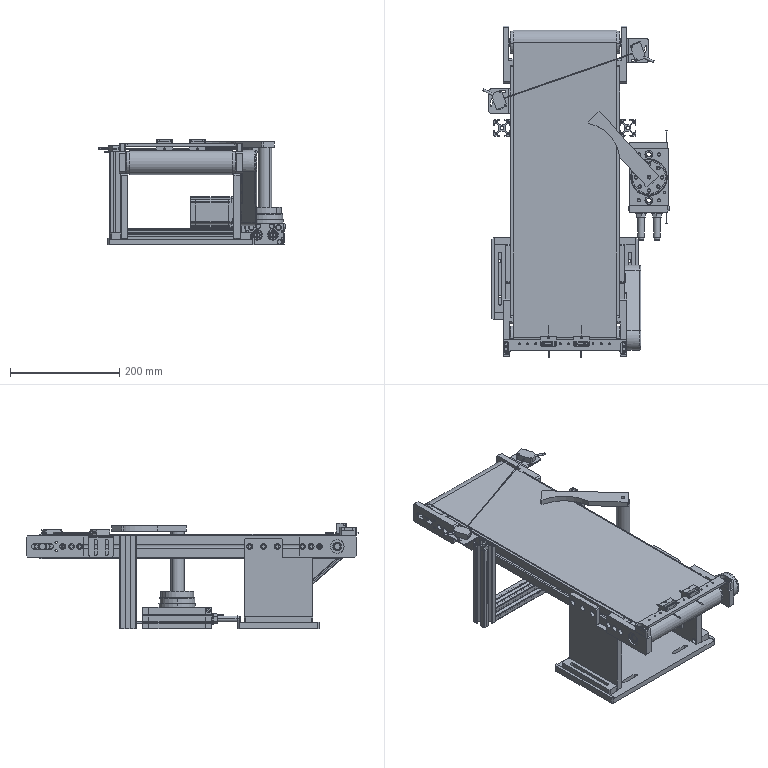Part | SolidWorks | features Belt 1 | 46 solids | 2799 faces | box 341.242 x 608 x 194 mm | volume 3807231 mm3 | cylinder 1354 | plane 1077 | cone 246 | spline 76 | torus 38 | sphere 8 | commonest cylinder face diameters 1.1 x110 0.5 x109 6.55 x98 6.6 x96 3 x62 4.2 x62